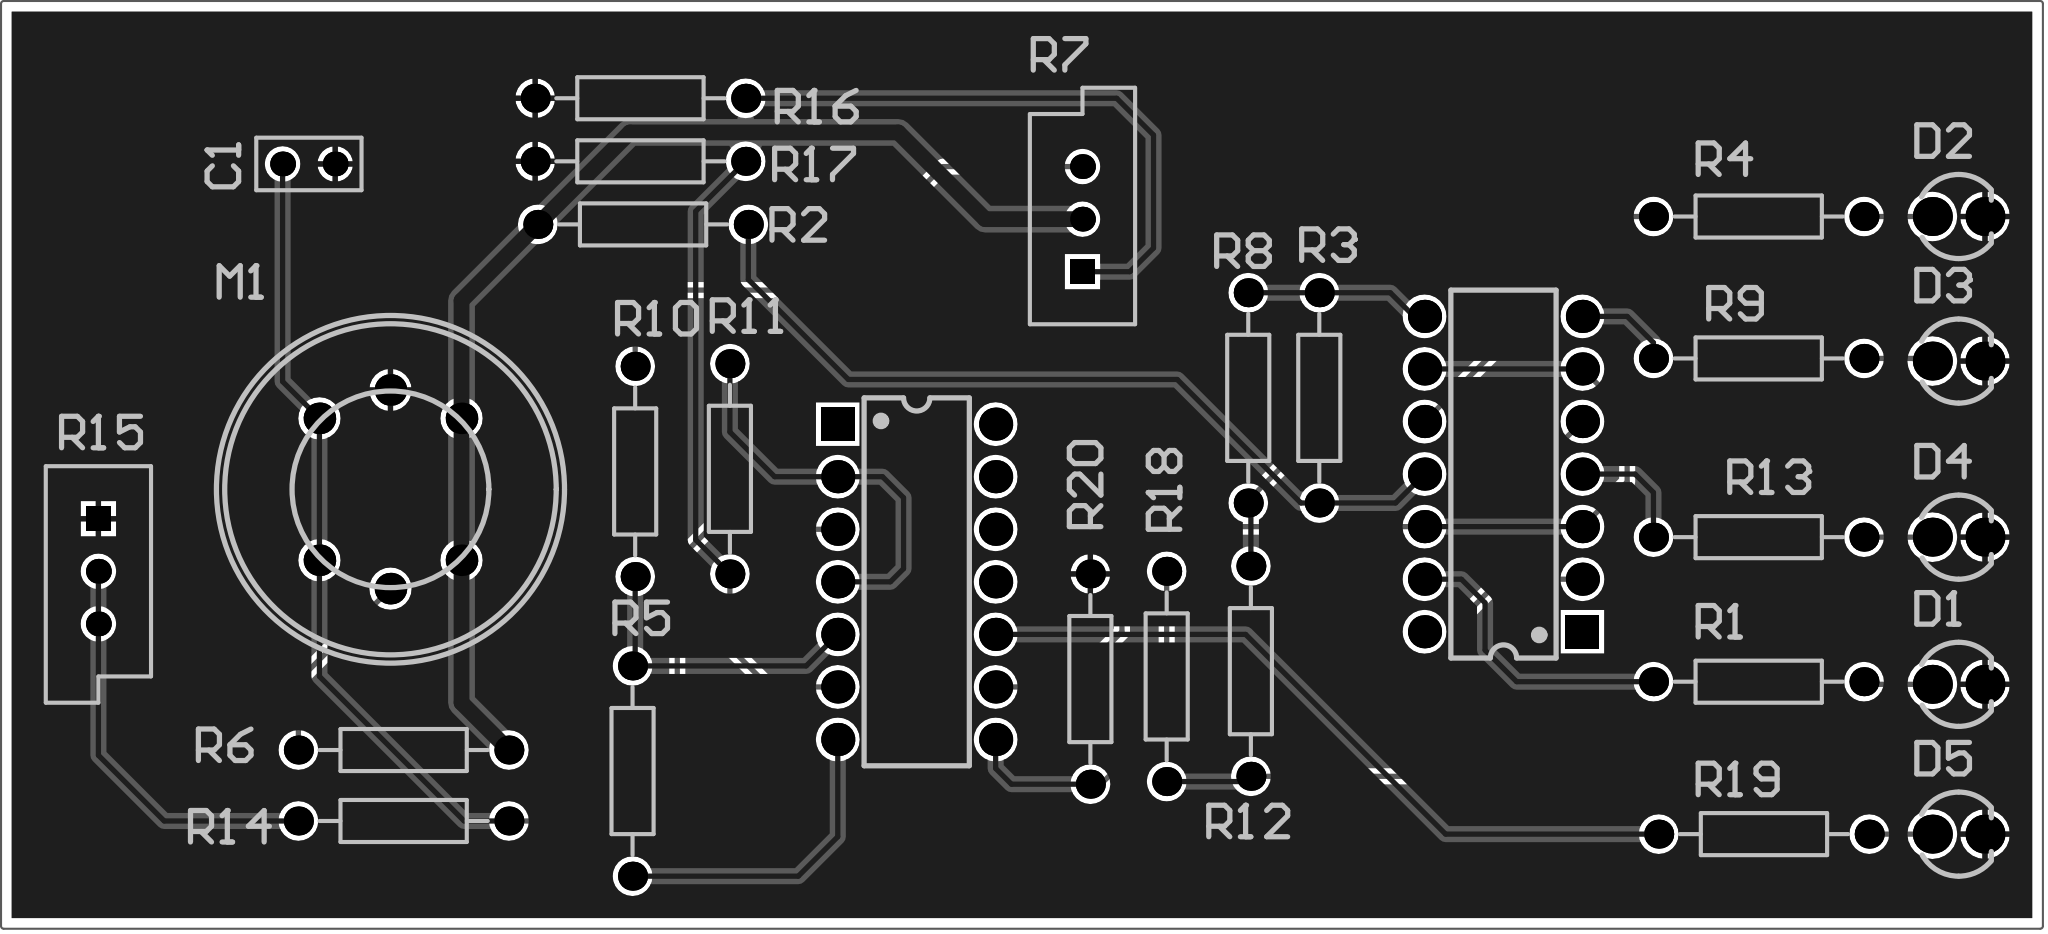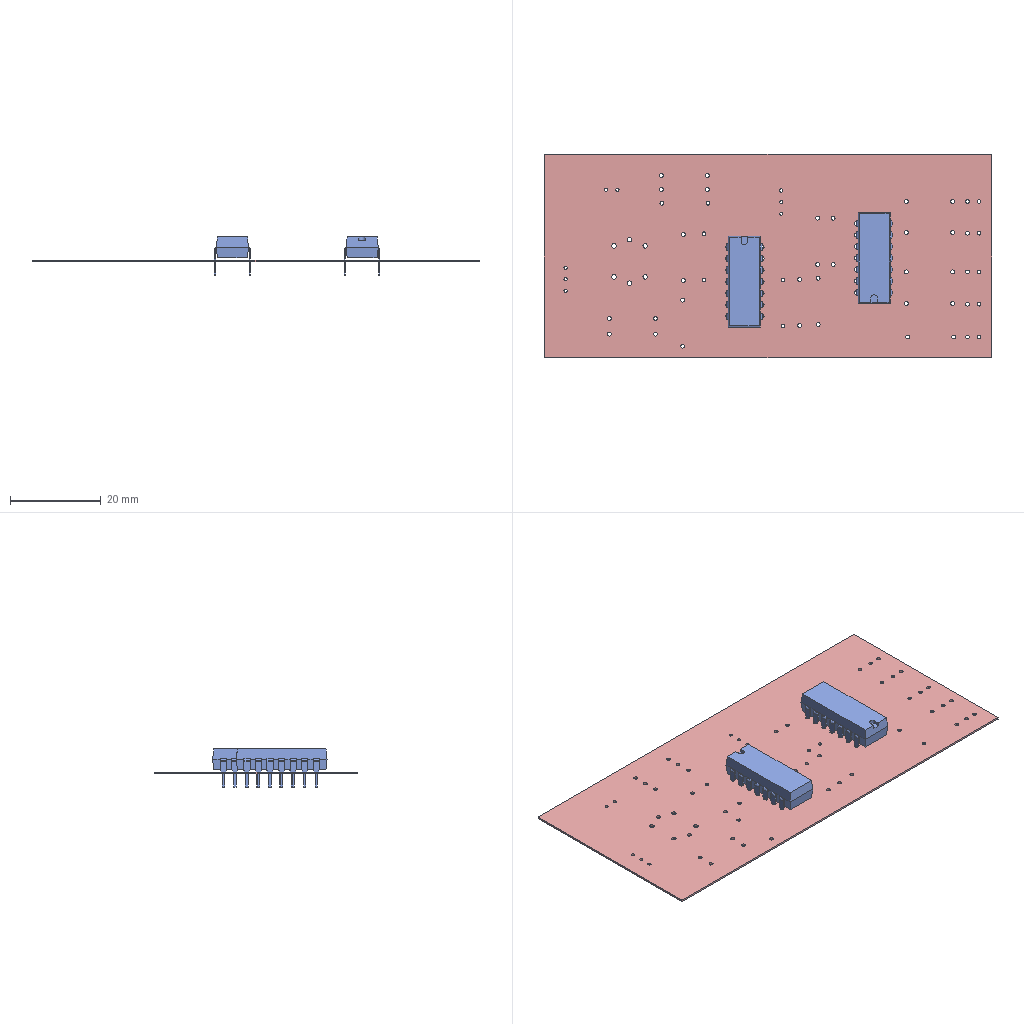Circuit board layout | Altium Designer | box 98.6 x 44.8 x 8.4 mm
Layer stack:
# Altium Designer layer stack of  (unit mm; dielectric type: 0 none, 1 core, 2 prepreg, 3 surface material)
index,name,kind,layer,copper_thickness_mm,dielectric_type,dielectric_thickness_mm,dielectric_material,dielectric_constant
0,Top Paste,other,,,,,,
1,Top Overlay,other,,,,,,
2,Top Solder,dielectric,,,3,0.0102,Solder Resist,3.5
3,Top Layer,copper,Top Layer,0.0356,,,,
4,Dielectric 1,dielectric,,,0,0.32,FR-4,4.8
5,Bottom Layer,copper,Bottom Layer,0.0356,,,,
6,Bottom Solder,dielectric,,,3,0.0102,Solder Resist,3.5
7,Bottom Overlay,other,,,,,,
8,Bottom Paste,other,,,,,,
# drill layer pairs: low layer,high layer
drill_pair,Top Layer,Bottom Layer
Part placement:
Designator,Comment,Layer,Footprint,Center-X(mm),Center-Y(mm),Rotation
R20,20K,TopLayer,AXIAL-0.4,90.678,48.133,90
R19,1K,TopLayer,AXIAL-0.4,123.19,40.64,360
R18,20K,TopLayer,AXIAL-0.4,94.361,48.26,90
R17,20K,TopLayer,AXIAL-0.4,68.961,73.152,360
R16,5.1K,TopLayer,AXIAL-0.4,68.961,76.2,360
R15,20K,TopLayer,VR5,42.799,53.34,270
R14,5.1K,TopLayer,AXIAL-0.4,57.531,41.275,360
R13,1K,TopLayer,AXIAL-0.4,122.936,54.991,360
R12,20K,TopLayer,AXIAL-0.4,98.425,48.514,270
R11,10K,TopLayer,AXIAL-0.4,73.279,58.293,90
R10,10K,TopLayer,AXIAL-0.4,68.707,58.166,90
R9,1K,TopLayer,AXIAL-0.4,122.936,63.627,360
R8,20K,TopLayer,AXIAL-0.4,98.298,61.722,270
R7,100K,TopLayer,VR5,90.297,70.358,90
R6,6.8,TopLayer,AXIAL-0.4,57.531,44.704,360
R5,20K,TopLayer,AXIAL-0.4,68.58,43.688,90
R4,1K,TopLayer,AXIAL-0.4,122.936,70.485,360
R3,20K,TopLayer,AXIAL-0.4,101.727,61.722,90
R2,200K,TopLayer,AXIAL-0.4,69.088,70.104,180
R1,1K,TopLayer,AXIAL-0.4,122.936,48.006,360
M1,MQ-2,TopLayer,MQ-2,56.896,57.303,0
D5,LED3,TopLayer,LED3MM,132.588,40.64,0
D4,LED3,TopLayer,LED3MM,132.588,54.991,0
D3,LED3,TopLayer,LED3MM,132.588,63.5,0
D2,LED3,TopLayer,LED3MM,132.588,70.485,0
D1,LED3,TopLayer,LED3MM,132.588,47.879,360
C1,0.1UF,TopLayer,RAD-0.1,52.959,73.025,180
*2,Component_1,TopLayer,DIP14,82.296,52.832,0
*1,Component_2,TopLayer,DIP14,110.617,58.039,180
Pad and via stacks:
# Altium Designer via and pad stacks of  (unit mm). Each distinct definition once, with the count of objects using it.
# via: kind,start_layer,end_layer,hole_mm,diameter_mm,mode(0 simple;1 top-mid-bottom;2 full stack),diameter_per_layer,count,example_net
# pad: kind,layer,hole_mm,hole_type(0 round;1 square;2 slot),plating,top_size,top_shape(1 round;2 rect;3 octagon;9 rounded rect),mid_size,bottom_size,mode,footprint,size_per_layer,count,example
pad,Multi-Layer,0.8128,2,plated,1.88x1.88,1,1.88x1.88,1.88x1.88,0,LED3MM,,10,D1.1
pad,Multi-Layer,0.85,0,plated,1.4x1.4,1,1.4x1.4,1.4x1.4,0,AXIAL-0.4,,36,R1.1
pad,Multi-Layer,0.7,0,plated,1.2x1.2,2,1.2x1.2,1.2x1.2,0,VR5,,2,R7.1
pad,Multi-Layer,0.7,0,plated,1.2x1.2,1,1.2x1.2,1.2x1.2,0,VR5,,4,R7.2
pad,Multi-Layer,0.8128,0,plated,1.6x1.6,1,1.6x1.6,1.6x1.6,0,DIP14,,26,*2.14
pad,Multi-Layer,0.8128,0,plated,1.6x1.6,2,1.6x1.6,1.6x1.6,0,DIP14,,2,*2.1
pad,Multi-Layer,1,0,plated,1.524x1.524,1,1.524x1.524,1.524x1.524,0,MQ-2,,6,M1.1
pad,Multi-Layer,0.7,0,plated,1.2x1.2,1,1.2x1.2,1.2x1.2,0,RAD-0.1,,2,C1.1
Copper pours:
name,layer,net,type(0 solid;1 hatched;2 none)
D,Top Layer,GND,0
D,Bottom Layer,GND,0
Design rules, without the lines most boards share:
# Altium Designer design rules of  (exported by Altium Designer, unit mm)
# columns: name | kind | enabled | priority | scope1 | scope2 | descriptor | typed fields (field=value)
Clearance | 0 | enabled | 1 | All | All | Clearance Constraint (Gap=10mil) (All),(All) | gap=0.254
PlaneConnect | 6 | enabled | 1 | All | All | Power Plane Connect Rule(Relief Connect )(Expansion=20mil) (Conductor Width=10mil) (Air Gap=10mil) (Entries=4) (All) | relief_conductor_width=0.254 relief_entries=4 relief_expansion=0.508
PolygonConnect | 20 | enabled | 1 | All | All | Polygon Connect Rule(Relief Connect )(Conductor Width=10mil) (Relief Angle=90 Angle) (Entries=4) (Air Gap Width=10mil) (All),(All) | connect_style(0=relief,1=direct,2=none)=0 relief_conductor_width=0.254 relief_entries=4
Width | 2 | enabled | 1 | All | All | Width Constraint (Min=10mil) (Max=30mil) (Preferred=10mil) (All) |
RoutingVias | 11 | enabled | 1 | All | All | Routing Via (MinHoleWidth=28mil) (MaxHoleWidth=28mil) (PreferredHoleWidth=28mil) (MinWidth=50mil) (MaxWidth=50mil) (PreferedWidth=50mil) (All) | via_min_hole=0.7112 via_max_hole=0.7112 via_preferred_diameter=1.27 via_preferred_hole=0.7112
PasteMaskExpansion | 14 | enabled | 1 | All | All | Paste Mask Expansion (Expansion =0mil) (All) | expansion=0
SolderMaskExpansion | 13 | enabled | 1 | All | All | Solder Mask Expansion (Expansion =4mil) (All) | expansion=0.1016
DiffPairsRouting | 51 | enabled | 1 | All | All | Differential Pairs Uncoupled Length using the Gap Constraints (Min=10mil) (Max=10mil) (Prefered=10mil)  and Width Constraints (Min=15mil) (Max=15mil) (Prefered=15mil) (All) |
HoleToHoleClearance | 52 | enabled | 1 | All | All | Hole To Hole Clearance (Gap=10mil) (All),(All) | gap=0.254
MinimumSolderMaskSliver | 53 | enabled | 1 | All | All | Minimum Solder Mask Sliver (Gap=0mil) (All),(All) |
SilkToSolderMaskClearance | 54 | enabled | 1 | IsPad | All | Silk To Solder Mask (Clearance=0mil) (IsPad),(All) |
SilkToSilkClearance | 55 | enabled | 1 | All | All | Silk to Silk (Clearance=0mil) (All),(All) |
Classes set for this board:
# Altium Designer classes of  (member kind: 0 net, 1 component, 2 from-to, 3 pad, 4 layer, 5 differential pair, 6 design channel, 7 polygon, 8 structure, 9 xSignal)
# columns: class name | member kind | superclass | members
Sheet1 | 1 | no | *1; *2; C1; D1; D2; D3; D4; D5; M1; R1; R2; R3; R4; R5; R6; R7; R8; R9; R10; R11; R12; R13; R14; R15; R16; R17; R18; R19; R20;